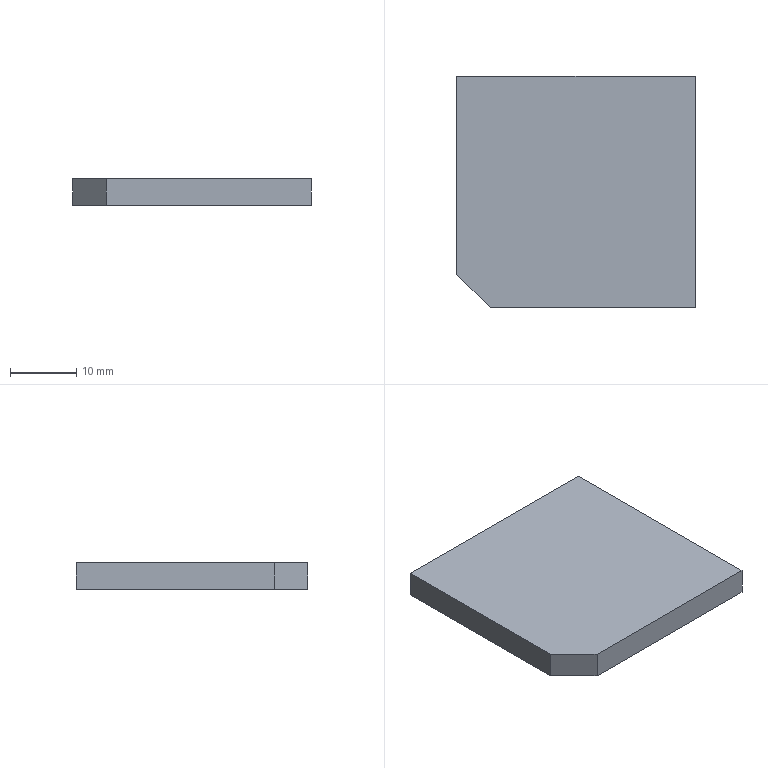Part | SolidWorks | features Chamfer 1, Extrusion 1 | 1 solid | 7 faces | box 36 x 35 x 4 mm | volume 4990 mm3 | plane 7
STEP:
#1=CARTESIAN_POINT('',(5.,0.,4.));
#2=VERTEX_POINT('',#1);
#3=CARTESIAN_POINT('',(36.,0.,4.));
#4=VERTEX_POINT('',#3);
#5=CARTESIAN_POINT('',(36.,0.,4.));
#6=DIRECTION('',(1.,0.,0.));
#7=VECTOR('',#6,1000.);
#8=LINE('',#5,#7);
#9=EDGE_CURVE('',#2,#4,#8,.T.);
#10=ORIENTED_EDGE('',*,*,#9,.F.);
#11=CARTESIAN_POINT('',(5.,0.,0.));
#12=VERTEX_POINT('',#11);
#13=CARTESIAN_POINT('',(5.,0.,4.));
#14=DIRECTION('',(0.,0.,-1.));
#15=VECTOR('',#14,1000.);
#16=LINE('',#13,#15);
#17=EDGE_CURVE('',#2,#12,#16,.T.);
#18=ORIENTED_EDGE('',*,*,#17,.T.);
#19=CARTESIAN_POINT('',(36.,0.,0.));
#20=VERTEX_POINT('',#19);
#21=CARTESIAN_POINT('',(36.,0.,0.));
#22=DIRECTION('',(1.,0.,0.));
#23=VECTOR('',#22,1000.);
#24=LINE('',#21,#23);
#25=EDGE_CURVE('',#12,#20,#24,.T.);
#26=ORIENTED_EDGE('',*,*,#25,.T.);
#27=CARTESIAN_POINT('',(36.,0.,4.));
#28=DIRECTION('',(0.,0.,-1.));
#29=VECTOR('',#28,1000.);
#30=LINE('',#27,#29);
#31=EDGE_CURVE('',#4,#20,#30,.T.);
#32=ORIENTED_EDGE('',*,*,#31,.F.);
#33=EDGE_LOOP('',(#10,#18,#26,#32));
#34=FACE_OUTER_BOUND('',#33,.T.);
#35=CARTESIAN_POINT('',(36.,0.,4.));
#36=DIRECTION('',(0.,1.,0.));
#37=DIRECTION('',(-1.,0.,0.));
#38=AXIS2_PLACEMENT_3D('',#35,#36,#37);
#39=PLANE('',#38);
#40=ADVANCED_FACE('',(#34),#39,.F.);
#41=CARTESIAN_POINT('',(36.,35.,0.));
#42=VERTEX_POINT('',#41);
#43=CARTESIAN_POINT('',(36.,35.,0.));
#44=DIRECTION('',(0.,1.,0.));
#45=VECTOR('',#44,1000.);
#46=LINE('',#43,#45);
#47=EDGE_CURVE('',#20,#42,#46,.T.);
#48=ORIENTED_EDGE('',*,*,#47,.T.);
#49=CARTESIAN_POINT('',(36.,35.,4.));
#50=VERTEX_POINT('',#49);
#51=CARTESIAN_POINT('',(36.,35.,4.));
#52=DIRECTION('',(0.,0.,-1.));
#53=VECTOR('',#52,1000.);
#54=LINE('',#51,#53);
#55=EDGE_CURVE('',#50,#42,#54,.T.);
#56=ORIENTED_EDGE('',*,*,#55,.F.);
#57=CARTESIAN_POINT('',(36.,35.,4.));
#58=DIRECTION('',(0.,1.,0.));
#59=VECTOR('',#58,1000.);
#60=LINE('',#57,#59);
#61=EDGE_CURVE('',#4,#50,#60,.T.);
#62=ORIENTED_EDGE('',*,*,#61,.F.);
#63=ORIENTED_EDGE('',*,*,#31,.T.);
#64=EDGE_LOOP('',(#48,#56,#62,#63));
#65=FACE_OUTER_BOUND('',#64,.T.);
#66=CARTESIAN_POINT('',(36.,35.,4.));
#67=DIRECTION('',(-1.,0.,0.));
#68=DIRECTION('',(0.,-1.,0.));
#69=AXIS2_PLACEMENT_3D('',#66,#67,#68);
#70=PLANE('',#69);
#71=ADVANCED_FACE('',(#65),#70,.F.);
#72=CARTESIAN_POINT('',(0.,35.,0.));
#73=VERTEX_POINT('',#72);
#74=CARTESIAN_POINT('',(0.,35.,0.));
#75=DIRECTION('',(-1.,0.,0.));
#76=VECTOR('',#75,1000.);
#77=LINE('',#74,#76);
#78=EDGE_CURVE('',#42,#73,#77,.T.);
#79=ORIENTED_EDGE('',*,*,#78,.T.);
#80=CARTESIAN_POINT('',(0.,35.,4.));
#81=VERTEX_POINT('',#80);
#82=CARTESIAN_POINT('',(0.,35.,4.));
#83=DIRECTION('',(0.,0.,-1.));
#84=VECTOR('',#83,1000.);
#85=LINE('',#82,#84);
#86=EDGE_CURVE('',#81,#73,#85,.T.);
#87=ORIENTED_EDGE('',*,*,#86,.F.);
#88=CARTESIAN_POINT('',(0.,35.,4.));
#89=DIRECTION('',(-1.,0.,0.));
#90=VECTOR('',#89,1000.);
#91=LINE('',#88,#90);
#92=EDGE_CURVE('',#50,#81,#91,.T.);
#93=ORIENTED_EDGE('',*,*,#92,.F.);
#94=ORIENTED_EDGE('',*,*,#55,.T.);
#95=EDGE_LOOP('',(#79,#87,#93,#94));
#96=FACE_OUTER_BOUND('',#95,.T.);
#97=CARTESIAN_POINT('',(0.,35.,4.));
#98=DIRECTION('',(0.,-1.,0.));
#99=DIRECTION('',(0.,0.,-1.));
#100=AXIS2_PLACEMENT_3D('',#97,#98,#99);
#101=PLANE('',#100);
#102=ADVANCED_FACE('',(#96),#101,.F.);
#103=CARTESIAN_POINT('',(0.,5.,0.));
#104=VERTEX_POINT('',#103);
#105=CARTESIAN_POINT('',(0.,0.,0.));
#106=DIRECTION('',(0.,-1.,0.));
#107=VECTOR('',#106,1000.);
#108=LINE('',#105,#107);
#109=EDGE_CURVE('',#73,#104,#108,.T.);
#110=ORIENTED_EDGE('',*,*,#109,.T.);
#111=CARTESIAN_POINT('',(0.,5.,4.));
#112=VERTEX_POINT('',#111);
#113=CARTESIAN_POINT('',(0.,5.,4.));
#114=DIRECTION('',(0.,0.,1.));
#115=VECTOR('',#114,1000.);
#116=LINE('',#113,#115);
#117=EDGE_CURVE('',#104,#112,#116,.T.);
#118=ORIENTED_EDGE('',*,*,#117,.T.);
#119=CARTESIAN_POINT('',(0.,0.,4.));
#120=DIRECTION('',(0.,-1.,0.));
#121=VECTOR('',#120,1000.);
#122=LINE('',#119,#121);
#123=EDGE_CURVE('',#81,#112,#122,.T.);
#124=ORIENTED_EDGE('',*,*,#123,.F.);
#125=ORIENTED_EDGE('',*,*,#86,.T.);
#126=EDGE_LOOP('',(#110,#118,#124,#125));
#127=FACE_OUTER_BOUND('',#126,.T.);
#128=CARTESIAN_POINT('',(0.,0.,4.));
#129=DIRECTION('',(1.,0.,0.));
#130=DIRECTION('',(0.,1.,0.));
#131=AXIS2_PLACEMENT_3D('',#128,#129,#130);
#132=PLANE('',#131);
#133=ADVANCED_FACE('',(#127),#132,.F.);
#134=ORIENTED_EDGE('',*,*,#123,.T.);
#135=CARTESIAN_POINT('',(5.,0.,4.));
#136=DIRECTION('',(0.7071,-0.7071,0.));
#137=VECTOR('',#136,1000.);
#138=LINE('',#135,#137);
#139=EDGE_CURVE('',#112,#2,#138,.T.);
#140=ORIENTED_EDGE('',*,*,#139,.T.);
#141=ORIENTED_EDGE('',*,*,#9,.T.);
#142=ORIENTED_EDGE('',*,*,#61,.T.);
#143=ORIENTED_EDGE('',*,*,#92,.T.);
#144=EDGE_LOOP('',(#134,#140,#141,#142,#143));
#145=FACE_OUTER_BOUND('',#144,.T.);
#146=CARTESIAN_POINT('',(0.,0.,4.));
#147=DIRECTION('',(0.,0.,-1.));
#148=DIRECTION('',(-1.,0.,0.));
#149=AXIS2_PLACEMENT_3D('',#146,#147,#148);
#150=PLANE('',#149);
#151=ADVANCED_FACE('',(#145),#150,.F.);
#152=ORIENTED_EDGE('',*,*,#25,.F.);
#153=CARTESIAN_POINT('',(2.5,2.5,0.));
#154=DIRECTION('',(-0.7071,0.7071,0.));
#155=VECTOR('',#154,1000.);
#156=LINE('',#153,#155);
#157=EDGE_CURVE('',#12,#104,#156,.T.);
#158=ORIENTED_EDGE('',*,*,#157,.T.);
#159=ORIENTED_EDGE('',*,*,#109,.F.);
#160=ORIENTED_EDGE('',*,*,#78,.F.);
#161=ORIENTED_EDGE('',*,*,#47,.F.);
#162=EDGE_LOOP('',(#152,#158,#159,#160,#161));
#163=FACE_OUTER_BOUND('',#162,.T.);
#164=CARTESIAN_POINT('',(0.,0.,0.));
#165=DIRECTION('',(0.,0.,-1.));
#166=DIRECTION('',(-1.,0.,0.));
#167=AXIS2_PLACEMENT_3D('',#164,#165,#166);
#168=PLANE('',#167);
#169=ADVANCED_FACE('',(#163),#168,.T.);
#170=ORIENTED_EDGE('',*,*,#139,.F.);
#171=ORIENTED_EDGE('',*,*,#117,.F.);
#172=ORIENTED_EDGE('',*,*,#157,.F.);
#173=ORIENTED_EDGE('',*,*,#17,.F.);
#174=EDGE_LOOP('',(#170,#171,#172,#173));
#175=FACE_OUTER_BOUND('',#174,.T.);
#176=CARTESIAN_POINT('',(5.,0.,4.));
#177=DIRECTION('',(0.7071,0.7071,0.));
#178=DIRECTION('',(0.,0.,-1.));
#179=AXIS2_PLACEMENT_3D('',#176,#177,#178);
#180=PLANE('',#179);
#181=ADVANCED_FACE('',(#175),#180,.F.);
#182=CLOSED_SHELL('',(#40,#71,#102,#133,#151,#169,#181));
#183=MANIFOLD_SOLID_BREP('',#182);
#184=CARTESIAN_POINT('',(0.,0.,0.));
#185=DIRECTION('',(0.,0.,1.));
#186=DIRECTION('',(1.,0.,0.));
#187=AXIS2_PLACEMENT_3D('',#184,#185,#186);
#188=(LENGTH_UNIT()NAMED_UNIT(*)SI_UNIT(.MILLI.,.METRE.));
#189=UNCERTAINTY_MEASURE_WITH_UNIT(LENGTH_MEASURE(0.00001),#188,'','');
#190=(NAMED_UNIT(*)PLANE_ANGLE_UNIT()SI_UNIT($,.RADIAN.));
#191=(NAMED_UNIT(*)SI_UNIT($,.STERADIAN.)SOLID_ANGLE_UNIT());
#192=(GEOMETRIC_REPRESENTATION_CONTEXT(3)GLOBAL_UNCERTAINTY_ASSIGNED_CONTEXT((#189))GLOBAL_UNIT_ASSIGNED_CONTEXT((#188,#190,#191))REPRESENTATION_CONTEXT('',''));
#193=ADVANCED_BREP_SHAPE_REPRESENTATION('',(#183,#187),#192);